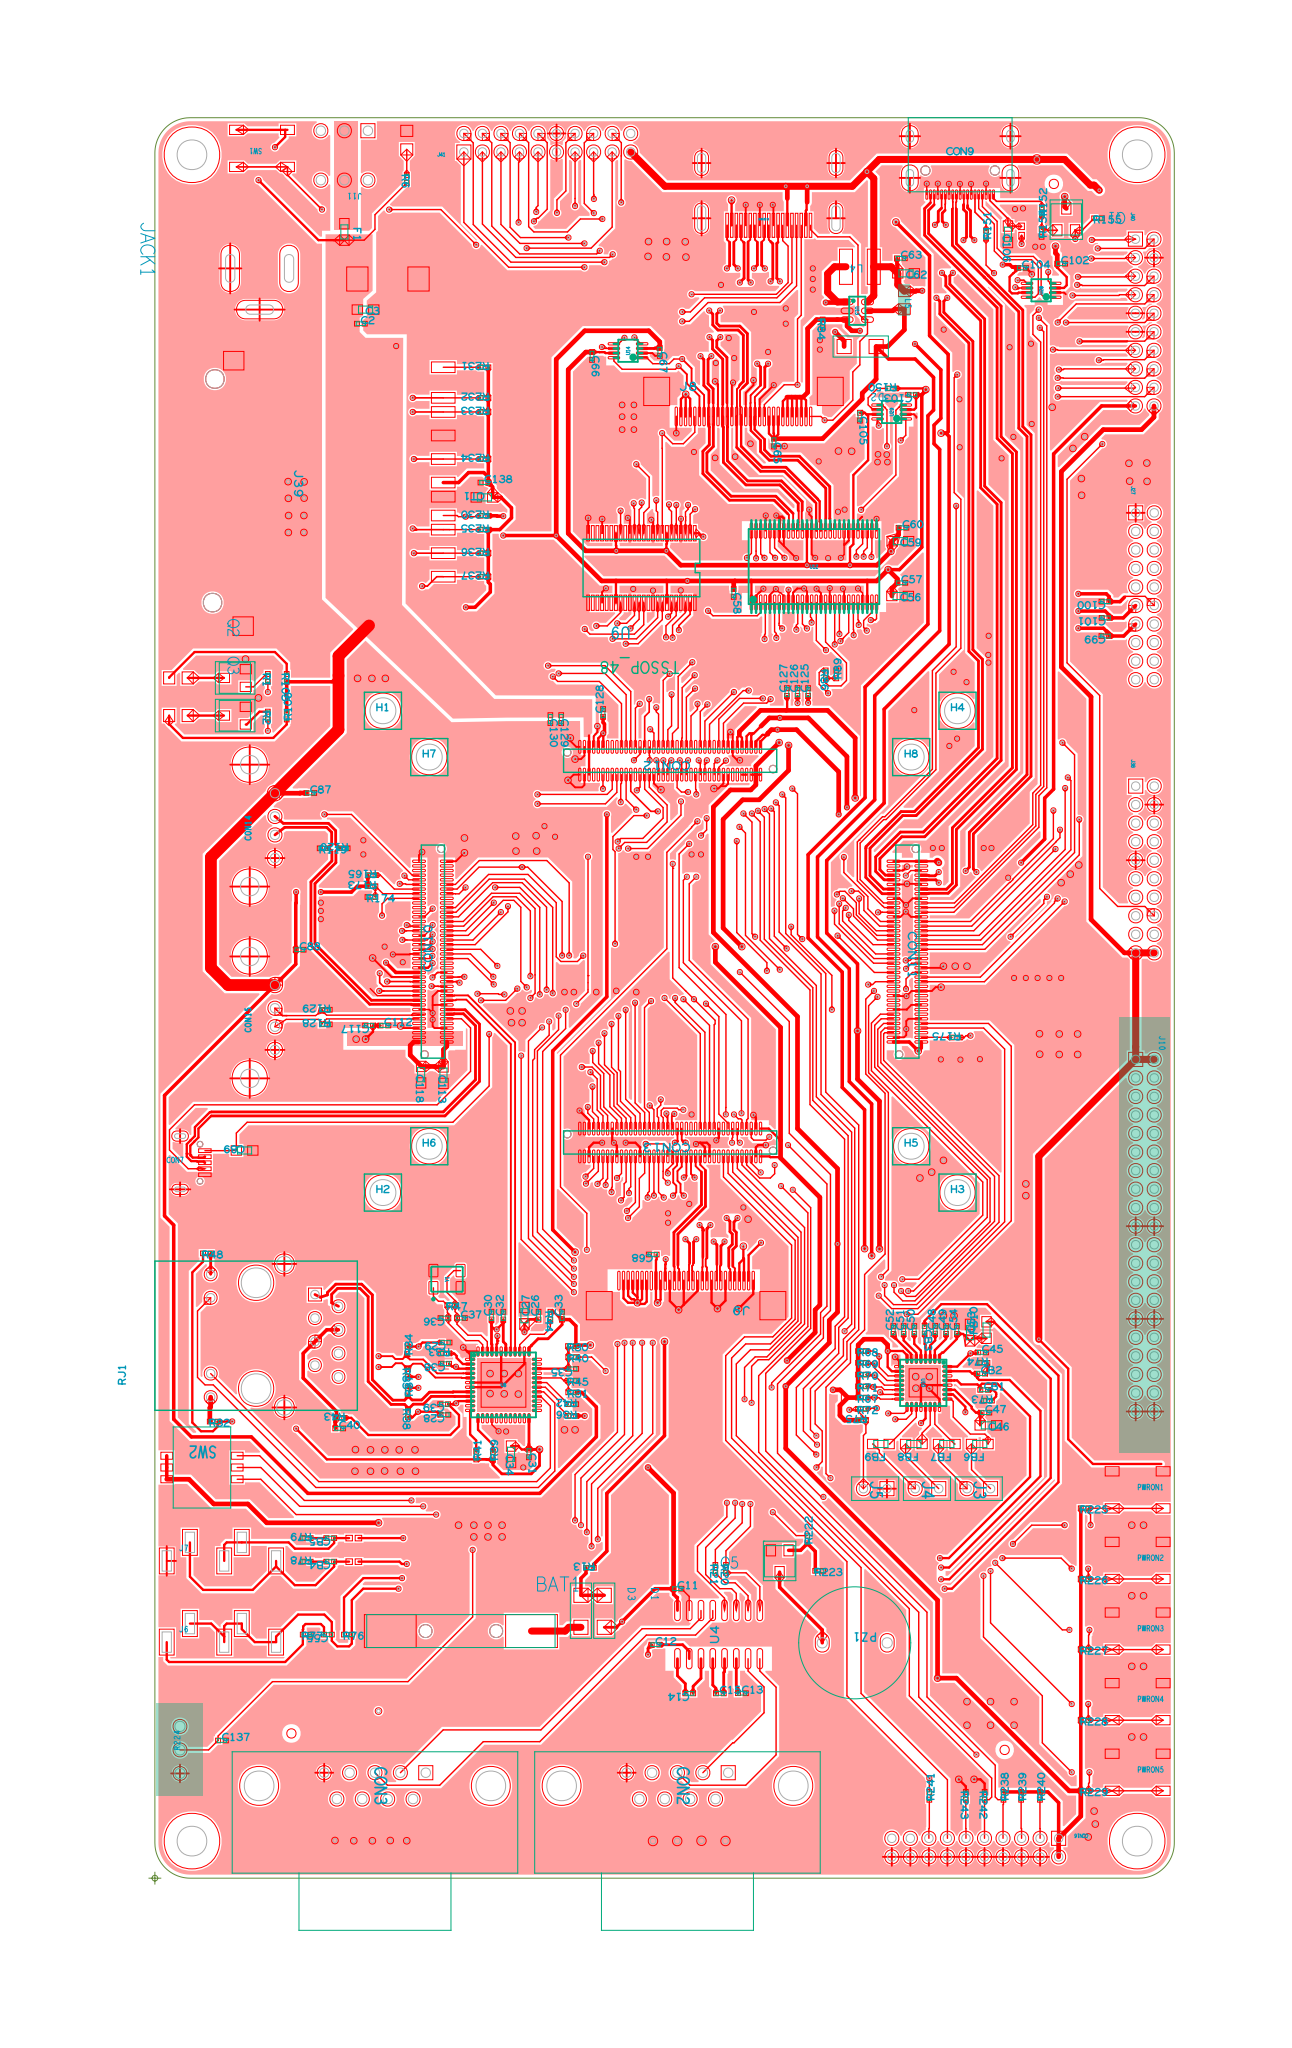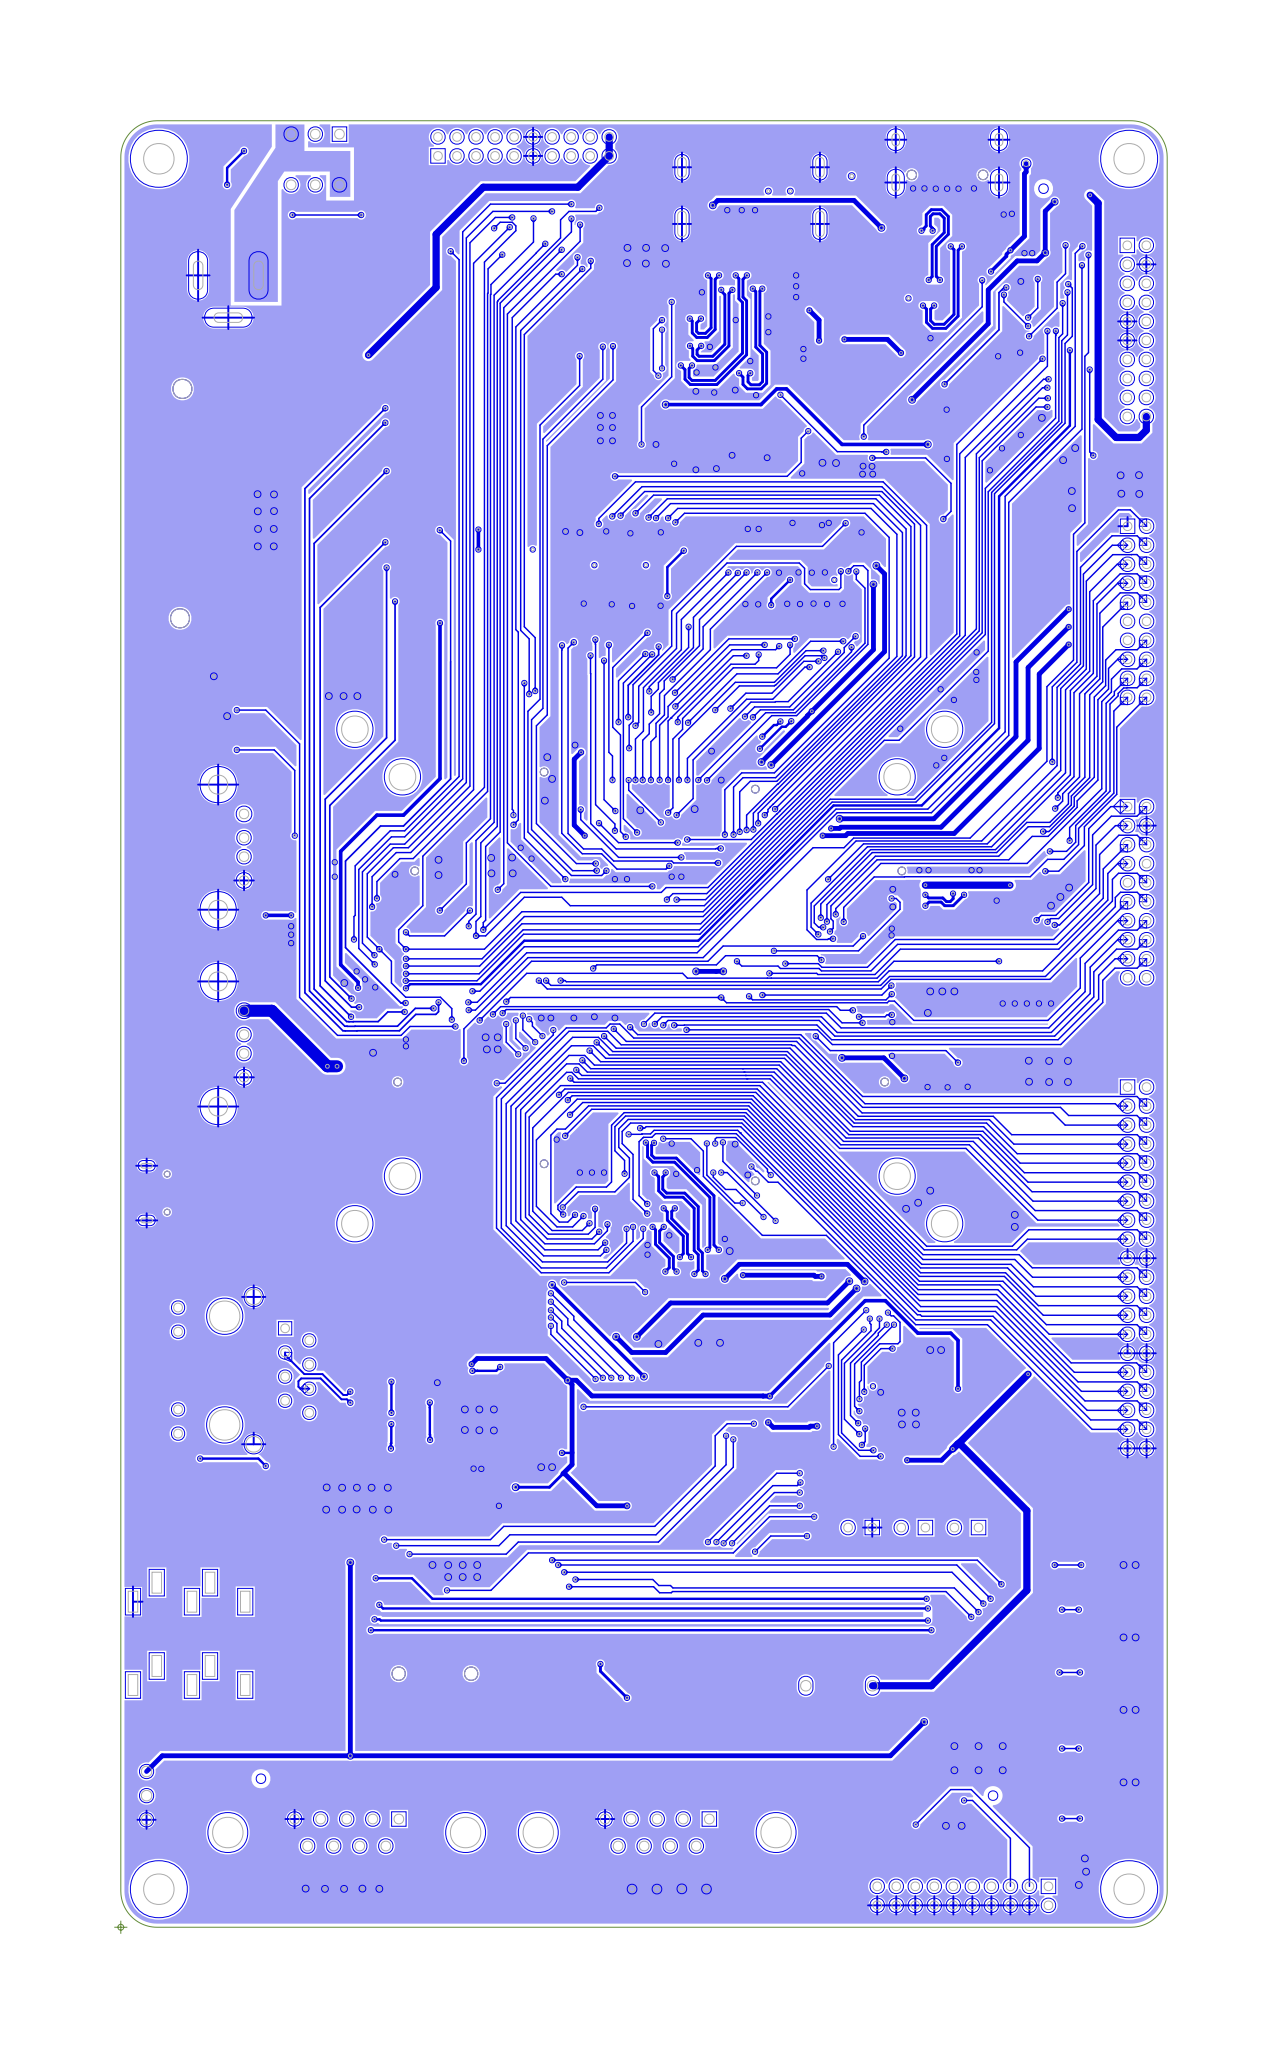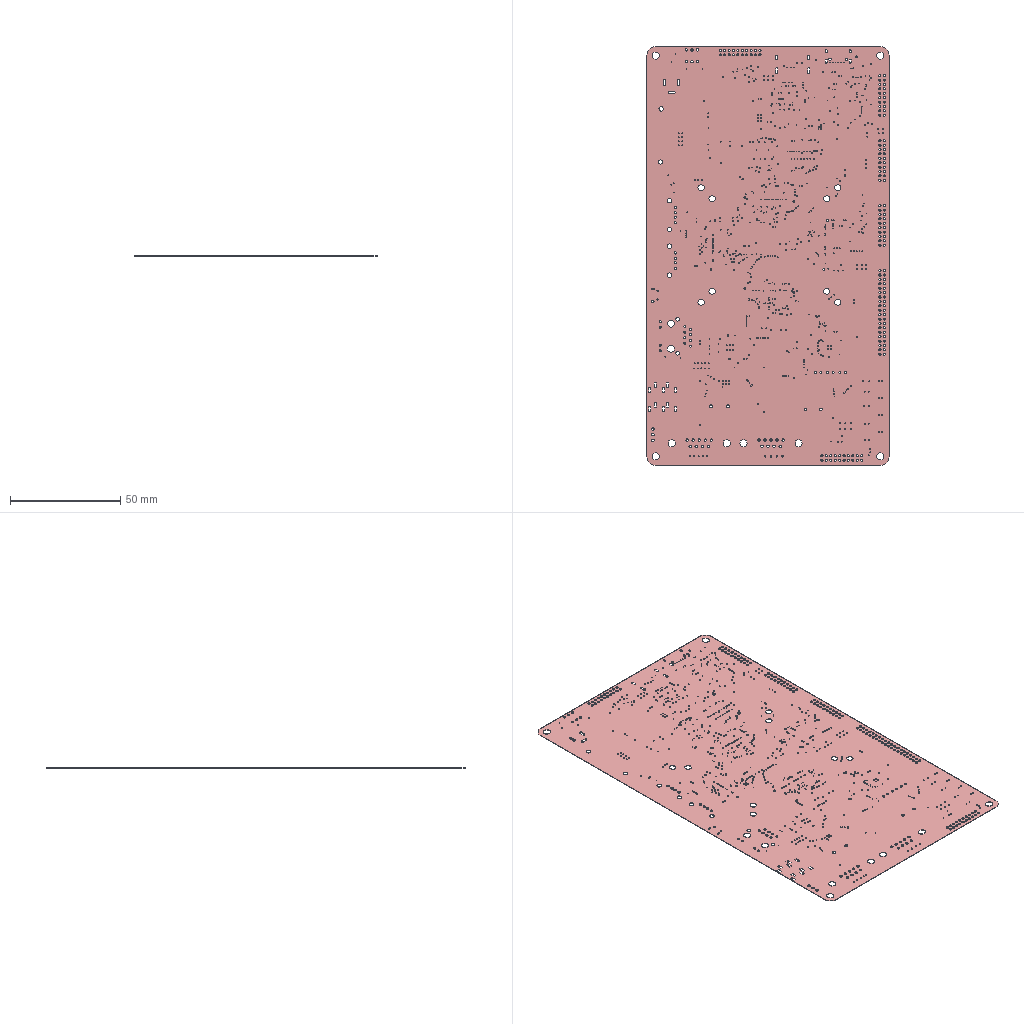Circuit board layout | Cadence Allegro | box 110 x 190 x 0.2 mm
Layer stack:
# Cadence Allegro layer stack of  (unit mm; from the constraint file cross-section; dielectric type: 0 not recorded (Allegro does not mark core vs prepreg), 3 surface material)
index,name,kind,layer,copper_thickness_mm,dielectric_type,dielectric_thickness_mm,dielectric_material,dielectric_constant
0,Top Surface,other,,,,,,
1,TOP,copper,TOP,0.0305,,,,
2,Dielectric1,dielectric,,,0,0.2032,FR-4,4.5
3,BOTTOM,copper,BOTTOM,0.0305,,,,
4,Bottom Surface,other,,,,,,
# drill layer pairs: low layer,high layer
drill_pair,TOP,BOTTOM
Part placement:
REFDES,COMP_VALUE,SYM_NAME,SYM_X,SYM_Y,SYM_ROTATE,SYM_MIRROR
BAT1,BATTERY,BAT1,1600.000,1050.000,0.000,NO
C1,100uF/16V,CT7343,990.000,6795.000,0.000,NO
C2,100nF,C0402,875.000,6605.000,0.000,NO
C3,10uF,C0603,895.000,6665.000,0.000,NO
C11,0.1uF,C0402,2220.000,1230.000,0.000,NO
C12,0.1uF,C0402,2127.000,992.000,0.000,NO
C13,0.1uF,C0402,2494.000,786.000,0.000,NO
C14,0.1uF,C0402,2270.000,785.000,180.000,NO
C15,0.1uF,C0402,2400.000,785.000,0.000,NO
C26,104,C0402,1630.000,2390.000,90.000,NO
C27,22uF/10V,C0603,1570.000,2390.000,90.000,NO
C28,104,C0402,1230.000,1969.000,180.000,NO
C29,104,C0402,1235.000,2276.000,180.000,NO
C30,104,C0402,1430.000,2390.000,90.000,NO
C31,104,C0402,1589.000,1805.000,270.000,NO
C32,104,C0402,1480.000,2390.000,90.000,NO
C33,104,C0402,1730.000,2390.000,90.000,NO
C34,22uF/10V,C0603,1513.000,1801.000,270.000,NO
C35,104,C0402,1772.957,2164.146,180.000,NO
C36,22pF,C0402,1230.000,2380.000,180.000,NO
C37,22pF,C0402,1300.000,2380.000,0.000,NO
C38,104,C0402,1233.000,2186.000,180.000,NO
C39,104,C0402,1229.000,2014.000,180.000,NO
C40,0.1uF,C0402,783.000,1911.000,0.000,NO
C45,2.2uF/16V,C0402,3514.000,2234.000,0.000,NO
C46,10uF/16V,C0603,3541.000,1924.000,0.000,NO
C47,100nF,C0402,3528.000,1978.000,0.000,NO
C48,1uF,C0402,3315.000,2330.000,90.000,NO
C49,1uF,C0402,3361.000,2329.000,90.000,NO
C50,1uF,C0402,3226.000,2329.000,90.000,NO
C51,1uF,C0402,3181.000,2329.000,90.000,NO
C52,1uF,C0402,3137.000,2329.000,90.000,NO
C53,10uF/16V,C0603,3463.000,2318.000,90.000,NO
C54,100nF,C0402,3407.000,2329.000,90.000,NO
C55,100pF,C0402,735.000,1035.000,180.000,NO
C56,10uF,C0603,3166.000,5448.000,0.000,NO
C57,100nF,C0402,3171.000,5504.000,0.000,NO
C58,100nF,C0402,2459.000,5461.000,270.000,NO
C59,10uF,C0603,3167.000,5681.000,0.000,NO
C60,100nF,C0402,3176.000,5738.000,0.000,NO
C62,10uF/16V,C0603,3191.000,6819.000,0.000,NO
C63,100nF,C0402,3169.000,6883.000,0.000,NO
C65,1uF/16V,C0402,2630.000,6100.000,270.000,NO
C66,0.1uF,C0402,1857.000,6468.000,270.000,NO
C67,0.1uF,C0402,2145.000,6485.000,270.000,NO
C68,1uF/16V,C0402,2115.000,2650.000,180.000,NO
C87,1uF/16V,C0402,660.000,4611.000,0.000,NO
C88,1uF/16V,C0402,615.000,3945.000,0.000,NO
C89,4.7uF,C0603,381.000,3092.000,180.000,NO
C99,2.2uF/16V,C0402,4038.000,5278.000,180.000,NO
C100,2.2uF/16V,C0402,4038.000,5424.000,180.000,NO
C101,2.2uF/16V,C0402,4039.000,5355.000,180.000,NO
C102,0.1uF,C0402,3850.000,6860.000,0.000,NO
C103,0.1uF,C0402,3217.000,6303.000,180.000,NO
C104,0.1uF,C0402,3684.000,6842.000,0.000,NO
C105,0.1uF,C0402,2995.000,6210.000,270.000,NO
C106,10uF,C0603,3624.000,6985.000,270.000,NO
C112,100nF,C0402,975.000,3623.000,0.000,NO
C113,22uF/10V,C0603,1226.000,3412.000,270.000,NO
C117,100nF,C0402,910.000,3623.000,180.000,NO
C118,22uF/10V,C0603,1131.000,3414.000,270.000,NO
C125,100nF,C0402,2775.000,5040.000,90.000,NO
C126,100nF,C0402,2730.000,5040.000,90.000,NO
C127,100nF,C0402,2685.000,5040.000,90.000,NO
C128,1uF/16V,C0402,1904.000,4951.000,90.000,NO
C129,100nF,C0402,1726.000,4925.000,270.000,NO
C130,100nF,C0402,1680.000,4925.000,270.000,NO
C137,100p,C0402,285.000,585.000,0.000,NO
C138,0.1uF,C0402,1400.000,5930.000,0.000,NO
CB1,100nF,C0402,3523.000,2075.000,0.000,NO
CB2,100nF,C0402,3510.000,2144.000,0.000,NO
CB3,1uF,C0402,3270.000,2330.000,270.000,NO
CB4,100nF,C0402,745.000,1345.000,180.000,NO
CB5,100nF,C0402,745.000,1445.000,180.000,NO
CON2,CON_DB9,DSUB9-RA-FE,2220.000,392.205,270.000,NO
CON3,CON_DB9,DSUB9-RA-FE,935.000,392.205,270.000,NO
CON6,hdmi19p,MD60-19P,2608.000,7053.000,180.000,NO
CON7,ZX62RD-AB-5P8,MICROUSB-B-H,50.000,3040.000,0.000,NO
CON9,MD60-19P,HDMI-C,3421.000,7323.000,0.000,NO
CON10,CON40X2_0_8MM,CON2X40-0_5MM-BB,1181.102,3937.008,90.000,NO
CON11,CON40X2_0_8MM,CON2X40-0_5MM-BB,3196.850,3937.008,270.000,NO
CON12,CON40X2_0_8MM,CON2X40-0_5MM-BB,2188.976,4748.031,180.000,NO
CON13,CON40X2_0_8MM,CON2X40-0_5MM-BB,2188.976,3125.984,180.000,NO
CON14,USB_A,USB-A2,510.000,4610.000,90.000,NO
CON15,USB_A,USB-A2,510.000,3795.000,90.000,NO
CON16,JTAG,HDRMS2MM-2X10,3485.000,130.000,180.000,NO
CT1,10uF/10V,C0603,1400.000,5867.000,180.000,NO
D1,IN4148,D1206,1909.000,1134.000,270.000,NO
D2,IN5819 NC,D1206,2996.000,6508.000,180.000,NO
D3,IN4148,D1206,1810.000,1134.000,270.000,NO
F1,YDQ,R0603,805.000,6995.000,270.000,NO
FB6,FB0603,FB0603,3504.224,1844.736,180.000,NO
FB7,FB0603,FB0603,3364.224,1844.736,180.000,NO
FB8,FB0603,FB0603,3224.224,1844.736,180.000,NO
FB9,FB0603,FB0603,3084.224,1844.736,180.000,NO
FB10,FB0603,FB0603,3533.000,2329.000,90.000,NO
FB17,BLM15AG221SN1D,L0402,3682.000,6999.000,90.000,NO
H1,TP_P0_0.8_D0,HOLE2_7,968.799,4960.413,0.000,NO
H2,TP_P0_0.8_D0,HOLE2_7,968.799,2913.169,0.000,NO
H3,TP_P0_0.8_D0,HOLE2_7,3409.744,2913.169,0.000,NO
H4,TP_P0_0.8_D0,HOLE2_7,3409.744,4960.413,0.000,NO
H5,TP_P0_0.8_D0,HOLE2_7,3212.906,3110.024,0.000,NO
H6,TP_P0_0.8_D0,HOLE2_7,1165.646,3110.024,0.000,NO
H7,TP_P0_0.8_D0,HOLE2_7,1165.646,4763.563,0.000,NO
H8,TP_P0_0.8_D0,HOLE2_7,3213.004,4763.563,0.000,NO
J3,CON2_2_54P,A4B-2PA-2_54DSA,3500.000,1655.000,270.000,NO
J4,CON2_2_54P,A4B-2PA-2_54DSA,3280.000,1655.000,270.000,NO
J5,CON2-2_54P,A4B-2PA-2_54DSA,3060.000,1655.000,270.000,NO
J6,JACK_AU,EAR_JACK,3.149,845.551,0.000,NO
J7,JACK_AU,EAR_JACK,3.149,1190.551,0.000,NO
J8,LVDS_QM,FPC30-050,2520.000,6211.000,0.000,NO
J9,LVDS_QM,FPC30-050,2237.000,2539.000,180.000,NO
J10,EBI Interface,HDRMS2MM-2X20,4166.700,3479.000,270.000,NO
J11,PS_L,SWITCH_DDSZ,905.000,7215.000,180.000,NO
J27,CON_CAMERA2M,HDRMS2MM-2X10,4206.100,5447.000,270.000,NO
J38,CON_GPIO,HDRMS2MM-2X10,4206.100,4286.000,270.000,NO
J39,SDCard,SDCARD,1225.000,6420.000,270.000,NO
J40,CON_GPIO,HDRMS2MM-2X10,4205.000,6610.000,270.000,NO
J41,CON_GPIO,HDRMS2MM-2X10,1667.000,7374.000,0.000,NO
JACK1,POWER JACK_3,JACK-2_5MM_B,570.000,6840.000,90.000,NO
L2,100nH,L0402,845.000,1345.000,0.000,NO
L3,100nH,L0402,845.000,1445.000,0.000,NO
L4,10uH NC,IND4018,2995.000,6847.000,180.000,NO
L5,1uH,R0805,3184.000,6705.000,270.000,NO
LED1,LED-Red (SMD 2012),LED-2012,1070.000,7385.000,90.000,NO
LED2,LED-Red (SMD 2012),LED-2012,100.000,5100.000,0.000,NO
LED3,LED-Red (SMD 2012),LED-2012,100.000,4940.000,0.000,NO
PWRON1,Home,SW4-SMD,4175.000,1650.000,0.000,NO
PWRON2,Back,SW4-SMD,4175.000,1350.000,0.000,NO
PWRON3,Sleep,SW4-SMD,4175.000,1050.000,0.000,NO
PWRON4,Vol+,SW4-SMD,4175.000,750.000,0.000,NO
PWRON5,Vol-,SW4-SMD,4175.000,450.000,0.000,NO
PZ1,PIEZO BUZZER_2,SPEAKER,3101.000,1000.000,180.000,NO
Q1,PDTC114YE,SOT-23,3872.000,7048.000,180.000,NO
Q2,L9014,SOT-23,340.000,5100.000,270.000,NO
Q3,L9014,SOT-23,340.000,4940.000,270.000,NO
Q5,L9014,SOT-23,2654.000,1347.000,0.000,NO
R1,1K,R0402,480.000,5100.000,270.000,NO
R2,1K,R0402,480.000,4940.000,270.000,NO
R6,10K,R0402,1070.000,7220.000,270.000,NO
R13,0R,R0402,1848.000,1319.000,180.000,NO
R20,0,R0402,2426.000,1314.000,270.000,NO
R21,0,R0402,2381.000,1314.000,270.000,NO
R30,10K/NC,R0402,1772.000,2261.000,0.000,NO
R31,10K,R0402,1772.957,2064.146,0.000,NO
R32,330R,R0402,250.000,1940.000,0.000,NO
R33,6.98K,R0402,1233.000,2230.000,180.000,NO
R34,49.9,R0402,1073.000,2243.000,90.000,NO
R35,49.9,R0402,1074.000,2147.000,270.000,NO
R36,10K,R0402,1772.957,1964.146,180.000,NO
R37,49.9,R0402,1074.000,2067.000,90.000,NO
R38,49.9,R0402,1075.000,1975.000,270.000,NO
R39,10K,R0402,1436.000,1795.000,90.000,NO
R40,0R,R0402,1772.957,2214.146,0.000,NO
R41,10K,R0402,1365.000,1796.000,90.000,NO
R42,10K,R0402,1772.957,2014.146,180.000,NO
R43,10.0,R0402,788.000,1956.000,180.000,NO
R44,10K,R0402,1680.000,2390.000,270.000,NO
R45,75K,R0402,1772.957,2114.146,0.000,NO
R47,1M,R0402,1259.000,2435.000,0.000,NO
R48,330R,R0402,221.000,2655.000,0.000,NO
R67,10K,R0402,3004.000,2042.000,0.000,NO
R68,10K,R0402,3004.224,2239.736,0.000,NO
R69,10K,R0402,3004.224,2189.736,0.000,NO
R70,10K,R0402,3004.224,2139.736,0.000,NO
R71,10K,R0402,3004.224,2089.736,0.000,NO
R72,0,R0402,3004.000,1994.000,0.000,NO
R73,20,R0402,3539.000,2029.000,180.000,NO
R74,20,R0402,3520.000,2190.000,180.000,NO
R75,10K,R0402,3004.000,1946.000,180.000,NO
R76,2.2K,R0402,820.000,1035.000,0.000,NO
R77,2.2K,R0402,645.000,1035.000,0.000,NO
R78,20R,R0402,645.000,1345.000,180.000,NO
R79,20R,R0402,645.000,1445.000,180.000,NO
R84,5R 1%,R0402,2837.000,6606.000,270.000,NO
R86,10K,R0402,2850.000,5115.000,270.000,NO
R89,N.M.,R0402,2895.000,5115.000,90.000,NO
R105,1K,R0402,560.000,5100.000,270.000,NO
R106,1K,R0402,560.000,4940.000,90.000,NO
R119,15K,R0402,717.000,4376.000,0.000,NO
R120,15K,R0402,802.000,4376.000,180.000,NO
R128,15K,R0402,726.000,3628.000,180.000,NO
R129,15K,R0402,726.000,3690.000,180.000,NO
R150,10K,R0402,3130.000,6330.000,180.000,NO
R151,33R,R0402,3531.000,6984.000,90.000,NO
R152,1K,R0402,3768.000,7083.000,90.000,NO
R154,47K,R0402,3767.000,6991.000,90.000,NO
R155,1K,R0402,4007.000,7053.000,0.000,NO
R165,800K,R0402,921.000,4262.000,180.000,NO
R173,800K(NC),R0402,920.000,4215.000,180.000,NO
R174,0,R0402,920.000,4169.000,0.000,NO
R175,NC,R0402,3402.000,3572.000,180.000,NO
R222,1K,R0402,2772.000,1439.000,90.000,NO
R223,10K,R0402,2822.000,1306.000,0.000,NO
R224,POT,SR2_54,106.575,445.000,90.000,NO
R225,10K,R0402,3950.000,1572.000,0.000,NO
R226,10K,R0402,3950.000,1271.000,0.000,NO
R227,10K,R0402,3950.000,972.000,0.000,NO
R228,10K,R0402,3950.000,671.000,0.000,NO
R229,10K,R0402,3950.000,371.000,0.000,NO
R230,10K,R0402,1400.000,5789.000,180.000,NO
R231,10K,R0402,1400.000,6420.000,180.000,NO
R232,10K,R0402,1400.000,6290.000,180.000,NO
R233,10K,R0402,1400.000,6230.000,180.000,NO
R234,10K,R0402,1400.000,6030.000,180.000,NO
R235,10K,R0402,1400.000,5730.000,180.000,NO
R236,10K,R0402,1400.000,5630.000,180.000,NO
R237,10K,R0402,1400.000,5530.000,180.000,NO
R238,NC,R0402,3605.000,350.000,90.000,NO
R239,NC,R0402,3680.000,350.000,90.000,NO
R240,NC,R0402,3760.000,350.000,90.000,NO
R241,NC,R0402,3290.000,350.000,90.000,NO
R242,NC,R0402,3525.000,350.000,270.000,NO
R243,0,R0402,3445.000,350.000,270.000,NO
RJ1,HR911105A,RJ8-SRLBY,430.000,2305.000,90.000,NO
SW1,RESET,SW4-SMD,455.000,7350.000,180.000,NO
SW2,SW-3,KHS03,200.000,1745.000,180.000,NO
U4,MAX3232CSE,SOIC16,2395.000,1035.000,90.000,NO
U8,DM9621NP,QFN48-050-0707LH,1481.000,2096.000,0.000,NO
U9,U-74ALVC164245DGG,TSSOP_48,2067.000,5567.000,180.000,NO
U10,WM8960GEFL,QFN32-050-5X5LH,3264.224,2104.736,270.000,NO
U12,SN75LVDS83BDGG,TSSOP56,2800.000,5573.000,0.000,NO
U13,TP3984,SOT23-6L,2984.000,6660.000,270.000,NO
U14,TXS0102DCU,TSSOP8,2010.000,6490.000,90.000,NO
U28,TXS0102DCU,TSSOP8,3765.000,6747.000,90.000,NO
U29,TXS0102DCU,TSSOP8,3130.000,6230.000,90.000,NO
Y1,25MHZ,X4-2_5X3_2,1240.957,2545.146,90.000,NO
Pad and via stacks, first 106 of 190 lines:
# Allegro (Cadence) via spans and padstacks; design units: ("mils" 3 1000)
# via spans: padstack,start_layer,end_layer,net_example,count
VIA12-Q,ETCH/TOP,ETCH/BOTTOM,GND,1
VIA12-BGA,ETCH/TOP,ETCH/BOTTOM,GND,40
VIA12-22BGA,ETCH/TOP,ETCH/BOTTOM,DC33V,611
VIA16-BGA,ETCH/TOP,ETCH/BOTTOM,GND,156
VIA24-Q,ETCH/TOP,ETCH/BOTTOM,GND,5
# Allegro padstack definitions: name,start_layer,end_layer,drill,plating,holeType,type
RX0_85Y2_70R0_10T,"ETCH/TOP","ETCH/TOP",0.0,"PLATED","none","smd"
SMD083X220,"ETCH/TOP","ETCH/TOP",0.0,"NON_PLATED","none","smd"
RX1_01Y3_49R0_10T,"ETCH/TOP","ETCH/TOP",0.0,"PLATED","none","smd"
RX10_77Y10_20R0_10T,"ETCH/TOP","ETCH/TOP",0.0,"PLATED","none","smd"
S2_3X2_6,"ETCH/TOP","ETCH/TOP",0.0,"NON_PLATED","none","smd"
S21X20,"ETCH/TOP","ETCH/TOP",0.0,"PLATED","none","smd"
SMD44X40,"ETCH/TOP","ETCH/TOP",0.0,"PLATED","none","smd"
SMD50X50,"ETCH/TOP","ETCH/TOP",0.0,"PLATED","none","smd"
SMT60X60,"ETCH/TOP","ETCH/TOP",0.0,"PLATED","none","smd"
S1_2X1_8,"ETCH/TOP","ETCH/TOP",0.0,"NON_PLATED","none","smd"
RX1_75Y2_40R0_10T,"ETCH/TOP","ETCH/TOP",0.0,"PLATED","none","smd"
SMD080X120,"ETCH/TOP","ETCH/TOP",0.0,"NON_PLATED","none","smd"
SMD010X080,"ETCH/TOP","ETCH/TOP",0.0,"PLATED","none","smd"
S1_35X0_4,"ETCH/TOP","ETCH/TOP",0.0,"NON_PLATED","none","smd"
SMD020X080,"ETCH/TOP","ETCH/TOP",0.0,"PLATED","none","smd"
SMD008X040,"ETCH/TOP","ETCH/TOP",0.0,"PLATED","none","smd"
SMD048X120,"ETCH/TOP","ETCH/TOP",0.0,"PLATED","none","smd"
SMD080X080,"ETCH/TOP","ETCH/TOP",0.0,"NON_PLATED","none","smd"
SMD016X048,"ETCH/TOP","ETCH/TOP",0.0,"PLATED","none","smd"
SMD012X040,"ETCH/TOP","ETCH/TOP",0.0,"PLATED","none","smd"
12X16SMD,"ETCH/TOP","ETCH/TOP",0.0,"NON_PLATED","none","smd"
24X28SMD,"ETCH/TOP","ETCH/TOP",0.0,"NON_PLATED","none","smd"
PAD1_2X1_4,"ETCH/TOP","ETCH/TOP",0.0,"NON_PLATED","none","smd"
S1_55X2_82,"ETCH/TOP","ETCH/TOP",0.0,"NON_PLATED","none","smd"
SMDR115X180,"ETCH/TOP","ETCH/TOP",0.0,"PLATED","none","smd"
S1_0X1_2,"ETCH/TOP","ETCH/TOP",0.0,"NON_PLATED","none","smd"
S0_7X0_6,"ETCH/TOP","ETCH/TOP",0.0,"NON_PLATED","none","smd"
91X20SMD,"ETCH/TOP","ETCH/TOP",0.0,"NON_PLATED","none","smd"
98X80SMD,"ETCH/TOP","ETCH/TOP",0.0,"NON_PLATED","none","smd"
76X80SMD,"ETCH/TOP","ETCH/TOP",0.0,"NON_PLATED","none","smd"
SMD047X087,"ETCH/TOP","ETCH/TOP",0.0,"NON_PLATED","none","smd"
SMD055X063,"ETCH/TOP","ETCH/TOP",0.0,"NON_PLATED","none","smd"
SMD047X055,"ETCH/TOP","ETCH/TOP",0.0,"NON_PLATED","none","smd"
SMD028X063,"ETCH/TOP","ETCH/TOP",0.0,"NON_PLATED","none","smd"
SMD060X095,"ETCH/TOP","ETCH/TOP",0.0,"NON_PLATED","none","smd"
SMD010X030,"ETCH/TOP","ETCH/TOP",0.0,"PLATED","none","smd"
SMD012X060,"ETCH/TOP","ETCH/TOP",0.0,"PLATED","none","smd"
SMD060X060,"ETCH/TOP","ETCH/TOP",0.0,"NON_PLATED","none","smd"
S1_4X3_8,"ETCH/TOP","ETCH/TOP",0.0,"NON_PLATED","none","smd"
S1_5X1_0,"ETCH/TOP","ETCH/TOP",0.0,"PLATED","none","smd"
14X20SMD,"ETCH/TOP","ETCH/TOP",0.0,"NON_PLATED","none","smd"
S1_27X0_76,"ETCH/TOP","ETCH/TOP",0.0,"PLATED","none","smd"
S0_8,"ETCH/TOP","ETCH/TOP",0.0,"NON_PLATED","none","smd"
SMDC100,"ETCH/TOP","ETCH/TOP",0.0,"PLATED","none","smd"
RX0_80Y0_45R0_10T,"ETCH/TOP","ETCH/TOP",0.0,"PLATED","none","smd"
SMD060X090,"ETCH/TOP","ETCH/TOP",0.0,"PLATED","none","smd"
SMD65_12,"ETCH/TOP","ETCH/TOP",0.0,"PLATED","none","smd"
OX0_25Y1_25T,"ETCH/TOP","ETCH/TOP",0.0,"PLATED","none","smd"
RX0_90Y0_30R0_10T,"ETCH/TOP","ETCH/TOP",0.0,"PLATED","none","smd"
BALL12,"ETCH/TOP","ETCH/TOP",0.0,"PLATED","none","smd"
OX0_27Y1_65T,"ETCH/TOP","ETCH/TOP",0.0,"PLATED","none","smd"
SMD010X040,"ETCH/TOP","ETCH/TOP",0.0,"PLATED","none","smd"
S0_4X0_8,"ETCH/TOP","ETCH/TOP",0.0,"NON_PLATED","none","smd"
OX0_60Y1_30T,"ETCH/TOP","ETCH/TOP",0.0,"PLATED","none","smd"
SMD15X70,"ETCH/TOP","ETCH/TOP",0.0,"PLATED","none","smd"
OX0_25Y1_10T,"ETCH/TOP","ETCH/TOP",0.0,"PLATED","none","smd"
RX0_30Y0_90R0_10T,"ETCH/TOP","ETCH/TOP",0.0,"PLATED","none","smd"
RX0_25Y0_40R0_10T,"ETCH/TOP","ETCH/TOP",0.0,"PLATED","none","smd"
SMD095X095,"ETCH/TOP","ETCH/TOP",0.0,"PLATED","none","smd"
SMD035X060,"ETCH/TOP","ETCH/TOP",0.0,"NON_PLATED","none","smd"
SMD070X098,"ETCH/TOP","ETCH/TOP",0.0,"NON_PLATED","none","smd"
SMD016X040,"ETCH/TOP","ETCH/TOP",0.0,"PLATED","none","smd"
SMD048X060,"ETCH/TOP","ETCH/TOP",0.0,"PLATED","none","smd"
SMD020X030,"ETCH/TOP","ETCH/TOP",0.0,"PLATED","none","smd"
SMD030X040,"ETCH/TOP","ETCH/TOP",0.0,"PLATED","none","smd"
RX1_35Y0_97R0_10T,"ETCH/TOP","ETCH/TOP",0.0,"PLATED","none","smd"
S0_4X1_0,"ETCH/TOP","ETCH/TOP",0.0,"NON_PLATED","none","smd"
SMD040X110,"ETCH/TOP","ETCH/TOP",0.0,"NON_PLATED","none","smd"
SMD024X085,"ETCH/TOP","ETCH/TOP",0.0,"PLATED","none","smd"
SMD012X020,"ETCH/TOP","ETCH/TOP",0.0,"PLATED","none","smd"
S0_65X1_0,"ETCH/TOP","ETCH/TOP",0.0,"NON_PLATED","none","smd"
SMD25_80,"ETCH/TOP","ETCH/TOP",0.0,"PLATED","none","smd"
S1_6X0_45,"ETCH/TOP","ETCH/TOP",0.0,"NON_PLATED","none","smd"
S1_6X0_3,"ETCH/TOP","ETCH/TOP",0.0,"NON_PLATED","none","smd"
S0_45X1_6,"ETCH/TOP","ETCH/TOP",0.0,"NON_PLATED","none","smd"
S0_3X1_6,"ETCH/TOP","ETCH/TOP",0.0,"NON_PLATED","none","smd"
SMD010X055,"ETCH/TOP","ETCH/TOP",0.0,"PLATED","none","smd"
S1_2X1_3,"ETCH/TOP","ETCH/TOP",0.0,"NON_PLATED","none","smd"
S0_7X0_5,"ETCH/TOP","ETCH/TOP",0.0,"NON_PLATED","none","smd"
FID10X20,"ETCH/TOP","ETCH/TOP",0.0,"PLATED","none","smd"
S1_3X1_3,"ETCH/TOP","ETCH/TOP",0.0,"NON_PLATED","none","smd"
SMD040X080,"ETCH/TOP","ETCH/TOP",0.0,"NON_PLATED","none","smd"
SMD040X070,"ETCH/TOP","ETCH/TOP",0.0,"NON_PLATED","none","smd"
SMD028X028,"ETCH/TOP","ETCH/TOP",0.0,"PLATED","none","smd"
S0_3,"ETCH/TOP","ETCH/TOP",0.0,"PLATED","none","smd"
SMD013X030,"ETCH/TOP","ETCH/TOP",0.0,"PLATED","none","smd"
S1_9X1_8,"ETCH/TOP","ETCH/TOP",0.0,"PLATED","none","smd"
SMD050X090,"ETCH/TOP","ETCH/TOP",0.0,"PLATED","none","smd"
SMDR220X60,"ETCH/TOP","ETCH/TOP",0.0,"PLATED","none","smd"
SMD220X140,"ETCH/TOP","ETCH/TOP",0.0,"PLATED","none","smd"
EX0_32Y0_32T,"ETCH/TOP","ETCH/TOP",0.0,"PLATED","none","smd"
SMD120X120,"ETCH/TOP","ETCH/TOP",0.0,"PLATED","none","smd"
SMDR200X220,"ETCH/TOP","ETCH/TOP",0.0,"PLATED","none","smd"
SMDR115X255,"ETCH/TOP","ETCH/TOP",0.0,"PLATED","none","smd"
S1_2X1_4,"ETCH/TOP","ETCH/TOP",0.0,"NON_PLATED","none","smd"
S1_1X1_9,"ETCH/TOP","ETCH/TOP",0.0,"NON_PLATED","none","smd"
SMD016X069,"ETCH/TOP","ETCH/TOP",0.0,"PLATED","none","smd"
S1_5X2_5,"ETCH/TOP","ETCH/TOP",0.0,"PLATED","none","smd"
Design rules, without the lines most boards share, first 14 of 116 lines:
# Cadence Allegro design rules of  (from the Constraint Manager export constraints.dcfx, design unit mil; typed fields in mm)
# columns: name | kind | enabled | priority | scope1 | scope2 | descriptor | typed fields (field=value)
# Allegro precedence (priority 1 wins): 1 Region class-to-class, 2 Region class, 3 Region, 4 class-to-class, 5 DiffPair/Bus/NetGroup override, 6 NetClass, 7 constraint set (CSet) default
# per-layer values are written LAYER=value in the descriptor and LAYER:mm in the typed field; a maximum of 0 means no limit set
# --- net classes (and buses / net groups) ---
SD | NetClass | enabled | 6 | XMMC2CLK, XMMC2CMD, XMMC2DATA0, XMMC2DATA1, XMMC2DATA2, XMMC2DATA3 | All | Net Class (members: 6 Net) overrides: (LINE_TO_LINE_SPACING=12mil) |  line_to_line_spacing=0.3048
XM0 | NetClass | enabled | 6 | XM0ADDR0, XM0ADDR1, XM0ADDR2, XM0ADDR3, XM0ADDR4, XM0ADDR5, XM0ADDR6, XM0ADDR7, XM0BEN0, XM0CS0, XM0CS1, XM0DATA_RDN, XM0DATA0, XM0DATA1, XM0DATA2, XM0DATA3, XM0DATA4, XM0DATA5, XM0DATA6, XM0DATA7, XM0DATA8, XM0DATA9, XM0DATA10, XM0DATA11, XM0DATA12, XM0DATA13, XM0DATA14, XM0DATA15, XM0OEN, XM0WEN | All | Net Class (members: 30 Net) overrides: (LINE_TO_LINE_SPACING=8mil) |  line_to_line_spacing=0.2032
PWR_PH | NetClass | enabled | 6 | DC33V | All | Net Class (members: 1 Net) overrides: (DIFFP_MIN_SPACE=5mil) |  diffp_min_space=0.127
# --- track widths, neck and differential-pair gap (physical constraint sets) ---
DEFAULT | PhysicalCSet | disabled (DRC mode MIN_LINE_WIDTH OFF) | 7 | Design default | All | Physical Constraint (Min Line Width=7mil) (Max Line Width=0mil) (Min Neck Width=5mil) (Max Neck Length=0mil) (DiffPair Primary Gap=0mil) (DiffPair Neck Gap=0mil) (DiffPair Min Space=0mil) (DiffPair Coupled +Tol=0mil) (DiffPair Coupled -Tol=0mil) (Min BB Via Stagger=5mil) (Max BB Via Stagger=0mil) (T-junctions=ANYWHERE) (Pad-pad direct connect=ALL_ALLOWED) (Allowed vias=VIA12-22BGA, VIA12-BGA, VIA16-Q, VIA24-Q, VIA02_04_BGA-Q, VIA12-Q) | min_line_width=0.1778 min_neck_width=0.127 min_bvia_stagger=0.127 max_bvia_stagger=0 ts_allowed=ANYWHERE diffp_primary_gap=0 diffp_neck_gap=0 max_line_width=0 maximum_neck_length=0 pad_pad_direct_connect=ALL_ALLOWED allow_on_etch_subclass=TRUE diffp_coupled_plus=0 diffp_coupled_minus=0 diffp_min_space=0 vias=VIA12-22BGA,VIA12-BGA,VIA16-Q,VIA24-Q,VIA02_04_BGA-Q,VIA12-Q
BGA-050 | PhysicalCSet | disabled (DRC mode MIN_LINE_WIDTH OFF) | 7 | not referenced | All | Physical Constraint (Min Line Width=4mil) (Max Line Width=0mil) (Min Neck Width=3mil) (Max Neck Length=0mil) (DiffPair Primary Gap=0mil) (DiffPair Neck Gap=0mil) (DiffPair Min Space=0mil) (DiffPair Coupled +Tol=0mil) (DiffPair Coupled -Tol=0mil) (Min BB Via Stagger=5mil) (Max BB Via Stagger=0mil) (T-junctions=ANYWHERE) (Pad-pad direct connect=ALL_ALLOWED) (Allowed vias=VIA12-22BGA) | min_line_width=0.1016 min_neck_width=0.0762 min_bvia_stagger=0.127 max_bvia_stagger=0 ts_allowed=ANYWHERE diffp_primary_gap=0 diffp_neck_gap=0 max_line_width=0 maximum_neck_length=0 pad_pad_direct_connect=ALL_ALLOWED allow_on_etch_subclass=TRUE diffp_coupled_plus=0 diffp_coupled_minus=0 diffp_min_space=0 vias=VIA12-22BGA
DIFF | PhysicalCSet | disabled (DRC mode MIN_LINE_WIDTH OFF) | 7 | Net(40): XMIPIMDN0, XMIPIMDN3, XMIPIMDP2, XMIPIMDPCLK, XMIPIMDP1, XMIPIMDP3, XMIPIMDN1, XMIPIMDP0, XMIPIMDNCLK, XMIPIMDN2, UH_DP3, XUOTGDP, ... | All | Physical Constraint (Min Line Width=6mil) (Max Line Width=0mil) (Min Neck Width=5mil) (Max Neck Length=0mil) (DiffPair Primary Gap=0mil) (DiffPair Neck Gap=0mil) (DiffPair Min Space=0mil) (DiffPair Coupled +Tol=0mil) (DiffPair Coupled -Tol=0mil) (Min BB Via Stagger=5mil) (Max BB Via Stagger=0mil) (T-junctions=ANYWHERE) (Pad-pad direct connect=ALL_ALLOWED) (Allowed vias=VIA12-BGA) | min_line_width=0.1524 min_neck_width=0.127 min_bvia_stagger=0.127 max_bvia_stagger=0 ts_allowed=ANYWHERE diffp_primary_gap=0 diffp_neck_gap=0 max_line_width=0 maximum_neck_length=0 pad_pad_direct_connect=ALL_ALLOWED allow_on_etch_subclass=TRUE diffp_coupled_plus=0 diffp_coupled_minus=0 diffp_min_space=0 vias=VIA12-BGA
# --- clearances: line / pad / via / shape / hole (spacing constraint sets) ---
RF1 | SpacingCSet | enabled | 7 | not referenced | All | Clearance Constraint (Line-Line=10mil) (Line-SMD Pad=6mil) (Line-Thru Pin=6mil) (Line-Via=6mil) (Line-Shape=20mil) (SMD Pad-SMD Pad=5mil) (Thru Pin-Thru Pin=0mil) (Thru Pin-SMD Pad=5mil) (SMD Pad-Via=5mil) (Thru Pin-Via=5mil) (Via-Via=5mil) (Shape-SMD Pad=8mil) (Shape-Thru Pin=8mil) (Shape-Via=8mil) (Shape-Shape=15mil) (Hole-Hole=0mil) (Hole-Line=8mil) (Hole-Shape=8mil) (BB Via-BB Via=5mil) (uVia-uVia=5mil) | thrupin_to_thrupin_spacing=0 thrupin_to_smdpin_spacing=0.127 thrupin_to_thruvia_spacing=0.127 line_to_thrupin_spacing=0.1524 thrupin_to_shape_spacing=0.2032 smdpin_to_smdpin_spacing=0.127 smdpin_to_thruvia_spacing=0.127 line_to_smdpin_spacing=0.1524 shape_to_smdpin_spacing=0.2032 thruvia_to_thruvia_spacing=0.127 line_to_thruvia_spacing=0.1524 shape_to_thruvia_spacing=0.2032 line_to_line_spacing=0.254 line_to_shape_spacing=0.508 shape_to_shape_spacing=0.381 bbv_to_bbv_spacing=0.127 bbv_to_thrupin_spacing=0.127 bbv_to_smdpin_spacing=0.127 bbv_to_thruvia_spacing=0.127 bbv_to_line_spacing=0.1524 bbv_to_shape_spacing=0.2032 bbv_to_testpin_spacing=0.127 bbv_to_testvia_spacing=0.127 testpin_to_testpin_spacing=0.127 testpin_to_thrupin_spacing=0.127 smdpin_to_testpin_spacing=0.127 testpin_to_thruvia_spacing=0.127 testpin_to_testvia_spacing=0.127 line_to_testpin_spacing=0.1524 shape_to_testpin_spacing=0.2032 testvia_to_testvia_spacing=0.127 testvia_to_thrupin_spacing=0.127 smdpin_to_testvia_spacing=0.127 testvia_to_thruvia_spacing=0.127 line_to_testvia_spacing=0.1524 shape_to_testvia_spacing=0.2032 bondpad_to_bondpad_spacing=0.127 thrupin_to_bondpad_spacing=0.127 smdpin_to_bondpad_spacing=0.127 bondpad_to_thruvia_spacing=0.127 bondpad_to_line_spacing=0.1524 bondpad_to_shape_spacing=0.2032 bondpad_to_bbv_spacing=0.127 bondpad_to_testpin_spacing=0.127 bondpad_to_testvia_spacing=0.127 min_bvia_gap=0.127 hole_to_pin_spacing=0.2029 hole_to_via_spacing=0.2029 hole_to_line_spacing=0.2032 hole_to_shape_spacing=0.2032 hole_to_hole_spacing=0 mvia_to_mvia_spacing=0.127 mvia_to_thrupin_spacing=0.127 mvia_to_smdpin_spacing=0.127 mvia_to_thruvia_spacing=0.127 mvia_to_bbv_spacing=0.127 mvia_to_line_spacing=0.1524 mvia_to_shape_spacing=0.2032 mvia_to_testpin_spacing=0.127 mvia_to_testvia_spacing=0.127 bondpad_to_mvia_spacing=0.127 bondpad_to_bondpad_diffp_spc=0.127